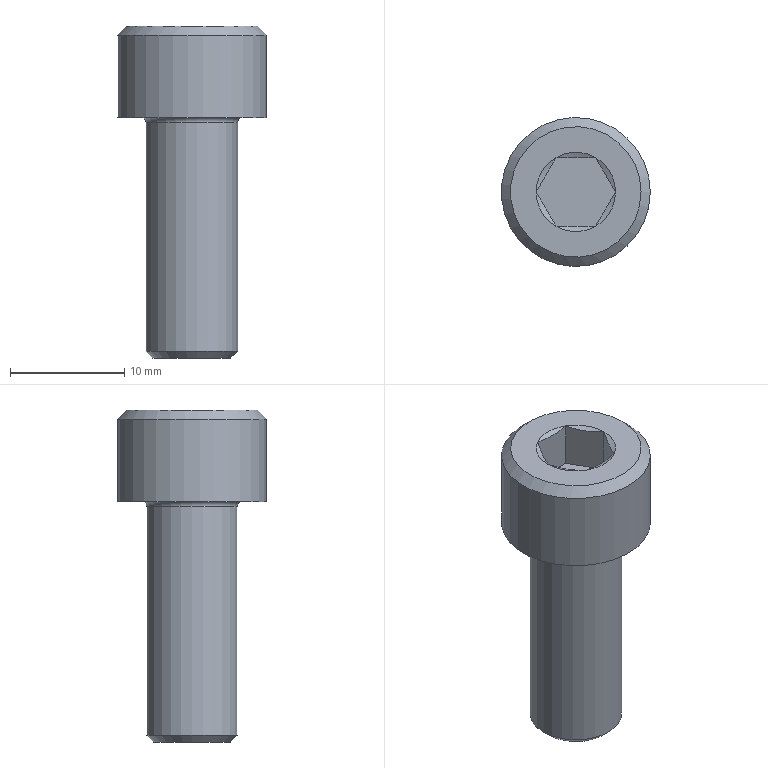Part | STEP file | solid 53 | 1 solid | 21 faces | box 13 x 13 x 29 mm | volume 1976 mm3 | plane 10 | sphere 6 | cylinder 2 | cone 2 | torus 1 | commonest cylinder face diameters 8 x1 13 x1